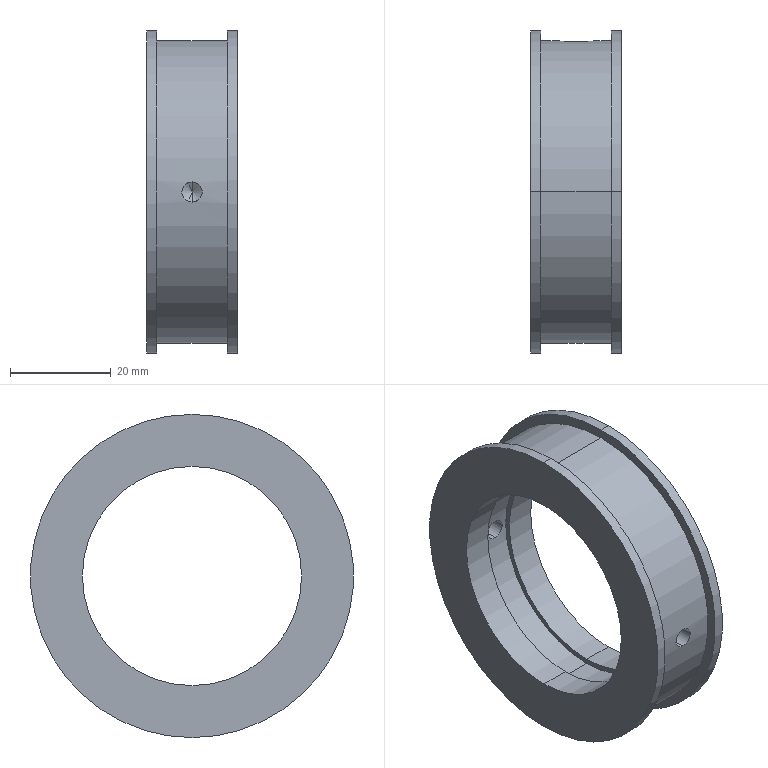Part | SolidWorks | features HoleWzd 3, Fillet 2, Revolution 1 | 1 solid | 31 faces | box 18 x 64 x 64 mm | volume 24795 mm3 | cylinder 18 | plane 7 | torus 2 | spline 2 | cone 2 | commonest cylinder face diameters 4 x4 43.4 x4 64 x4 7.5 x2 45.4 x2 60 x2
STEP:
#1=CARTESIAN_POINT('',(0.6103,28.8,3.75));
#2=VERTEX_POINT('',#1);
#3=CARTESIAN_POINT('',(0.6103,28.8,-3.75));
#4=VERTEX_POINT('',#3);
#5=CARTESIAN_POINT('',(0.6103,28.8,0.));
#6=DIRECTION('',(0.,-1.,0.));
#7=DIRECTION('',(0.,0.,-1.));
#8=AXIS2_PLACEMENT_3D('',#5,#6,#7);
#9=CIRCLE('',#8,3.75);
#10=EDGE_CURVE('',#2,#4,#9,.T.);
#11=ORIENTED_EDGE('',*,*,#10,.F.);
#12=CARTESIAN_POINT('',(0.6103,28.5,3.45));
#13=VERTEX_POINT('',#12);
#14=CARTESIAN_POINT('',(0.6103,28.8,3.45));
#15=DIRECTION('',(1.,0.,0.));
#16=DIRECTION('',(0.,0.,-1.));
#17=AXIS2_PLACEMENT_3D('',#14,#15,#16);
#18=CIRCLE('',#17,0.3);
#19=EDGE_CURVE('',#2,#13,#18,.T.);
#20=ORIENTED_EDGE('',*,*,#19,.T.);
#21=CARTESIAN_POINT('',(0.6103,28.5,-3.45));
#22=VERTEX_POINT('',#21);
#23=CARTESIAN_POINT('',(0.6103,28.5,0.));
#24=DIRECTION('',(0.,1.,0.));
#25=DIRECTION('',(0.,0.,-1.));
#26=AXIS2_PLACEMENT_3D('',#23,#24,#25);
#27=CIRCLE('',#26,3.45);
#28=EDGE_CURVE('',#22,#13,#27,.T.);
#29=ORIENTED_EDGE('',*,*,#28,.F.);
#30=CARTESIAN_POINT('',(0.6103,28.8,-3.45));
#31=DIRECTION('',(-1.,0.,0.));
#32=DIRECTION('',(0.,0.,1.));
#33=AXIS2_PLACEMENT_3D('',#30,#31,#32);
#34=CIRCLE('',#33,0.3);
#35=EDGE_CURVE('',#4,#22,#34,.T.);
#36=ORIENTED_EDGE('',*,*,#35,.F.);
#37=EDGE_LOOP('',(#11,#20,#29,#36));
#38=FACE_OUTER_BOUND('',#37,.T.);
#39=CARTESIAN_POINT('',(0.6103,28.8,0.));
#40=DIRECTION('',(0.,-1.,0.));
#41=DIRECTION('',(0.,0.,-1.));
#42=AXIS2_PLACEMENT_3D('',#39,#40,#41);
#43=TOROIDAL_SURFACE('',#42,3.45,0.3);
#44=ADVANCED_FACE('',(#38),#43,.F.);
#45=CARTESIAN_POINT('',(-0.2424,29.551,-3.652));
#46=VERTEX_POINT('',#45);
#47=CARTESIAN_POINT('',(0.6103,29.537,3.75));
#48=VERTEX_POINT('',#47);
#49=CARTESIAN_POINT('',(-0.2424,29.551,-3.652));
#50=CARTESIAN_POINT('',(-0.4646,29.558,-3.6));
#51=CARTESIAN_POINT('',(-0.6839,29.568,-3.527));
#52=CARTESIAN_POINT('',(-1.101,29.591,-3.345));
#53=CARTESIAN_POINT('',(-1.299,29.605,-3.236));
#54=CARTESIAN_POINT('',(-1.675,29.634,-2.982));
#55=CARTESIAN_POINT('',(-1.854,29.65,-2.836));
#56=CARTESIAN_POINT('',(-2.178,29.682,-2.518));
#57=CARTESIAN_POINT('',(-2.324,29.698,-2.346));
#58=CARTESIAN_POINT('',(-2.586,29.728,-1.974));
#59=CARTESIAN_POINT('',(-2.701,29.742,-1.774));
#60=CARTESIAN_POINT('',(-2.891,29.766,-1.363));
#61=CARTESIAN_POINT('',(-2.967,29.776,-1.149));
#62=CARTESIAN_POINT('',(-3.08,29.792,-0.7059));
#63=CARTESIAN_POINT('',(-3.116,29.797,-0.479));
#64=CARTESIAN_POINT('',(-3.146,29.801,-0.02683));
#65=CARTESIAN_POINT('',(-3.141,29.8,0.2003));
#66=CARTESIAN_POINT('',(-3.089,29.793,0.6567));
#67=CARTESIAN_POINT('',(-3.042,29.786,0.8794));
#68=CARTESIAN_POINT('',(-2.91,29.769,1.312));
#69=CARTESIAN_POINT('',(-2.823,29.757,1.524));
#70=CARTESIAN_POINT('',(-2.613,29.731,1.93));
#71=CARTESIAN_POINT('',(-2.491,29.717,2.121));
#72=CARTESIAN_POINT('',(-2.213,29.686,2.478));
#73=CARTESIAN_POINT('',(-2.056,29.67,2.647));
#74=CARTESIAN_POINT('',(-1.716,29.638,2.95));
#75=CARTESIAN_POINT('',(-1.534,29.623,3.084));
#76=CARTESIAN_POINT('',(-1.147,29.594,3.32));
#77=CARTESIAN_POINT('',(-0.9399,29.581,3.422));
#78=CARTESIAN_POINT('',(-0.5152,29.56,3.584));
#79=CARTESIAN_POINT('',(-0.2972,29.552,3.646));
#80=CARTESIAN_POINT('',(0.1503,29.54,3.729));
#81=CARTESIAN_POINT('',(0.3805,29.537,3.75));
#82=CARTESIAN_POINT('',(0.6103,29.537,3.75));
#83=B_SPLINE_CURVE_WITH_KNOTS('',3,(#49,#50,#51,#52,#53,#54,#55,#56,#57,#58,#59,#60,#61,#62,#63,#64,#65,#66,#67,#68,#69,#70,#71,#72,#73,#74,#75,#76,#77,#78,#79,#80,#81,#82),.UNSPECIFIED.,.F.,.F.,(4,2,2,2,2,2,2,2,2,2,2,2,2,2,2,2,4),(0.01269,0.01337,0.01406,0.01474,0.01543,0.01611,0.0168,0.01748,0.01817,0.01885,0.01954,0.02022,0.02091,0.02159,0.02228,0.02296,0.02365),.UNSPECIFIED.);
#84=EDGE_CURVE('',#46,#48,#83,.T.);
#85=ORIENTED_EDGE('',*,*,#84,.F.);
#86=CARTESIAN_POINT('',(-0.2879,29.749,-3.872));
#87=VERTEX_POINT('',#86);
#88=CARTESIAN_POINT('',(-0.2879,29.551,-3.847));
#89=DIRECTION('',(-0.9734,0.02959,0.2273));
#90=DIRECTION('',(0.2274,0.,0.9738));
#91=AXIS2_PLACEMENT_3D('',#88,#89,#90);
#92=CIRCLE('',#91,0.2);
#93=EDGE_CURVE('',#46,#87,#92,.T.);
#94=ORIENTED_EDGE('',*,*,#93,.T.);
#95=CARTESIAN_POINT('',(1.509,29.749,3.872));
#96=VERTEX_POINT('',#95);
#97=CARTESIAN_POINT('',(1.509,29.749,3.872));
#98=CARTESIAN_POINT('',(1.254,29.741,3.932));
#99=CARTESIAN_POINT('',(0.9958,29.737,3.966));
#100=CARTESIAN_POINT('',(0.4738,29.734,3.983));
#101=CARTESIAN_POINT('',(0.2098,29.737,3.965));
#102=CARTESIAN_POINT('',(-0.3023,29.748,3.878));
#103=CARTESIAN_POINT('',(-0.5513,29.757,3.81));
#104=CARTESIAN_POINT('',(-1.035,29.78,3.624));
#105=CARTESIAN_POINT('',(-1.271,29.795,3.506));
#106=CARTESIAN_POINT('',(-1.707,29.826,3.231));
#107=CARTESIAN_POINT('',(-1.911,29.843,3.072));
#108=CARTESIAN_POINT('',(-2.289,29.878,2.714));
#109=CARTESIAN_POINT('',(-2.459,29.895,2.517));
#110=CARTESIAN_POINT('',(-2.756,29.927,2.096));
#111=CARTESIAN_POINT('',(-2.886,29.943,1.869));
#112=CARTESIAN_POINT('',(-3.098,29.969,1.394));
#113=CARTESIAN_POINT('',(-3.18,29.979,1.149));
#114=CARTESIAN_POINT('',(-3.296,29.994,0.6447));
#115=CARTESIAN_POINT('',(-3.33,29.999,0.3829));
#116=CARTESIAN_POINT('',(-3.346,30.001,-0.135));
#117=CARTESIAN_POINT('',(-3.329,29.999,-0.3927));
#118=CARTESIAN_POINT('',(-3.245,29.987,-0.9056));
#119=CARTESIAN_POINT('',(-3.177,29.979,-1.16));
#120=CARTESIAN_POINT('',(-2.996,29.956,-1.643));
#121=CARTESIAN_POINT('',(-2.882,29.942,-1.876));
#122=CARTESIAN_POINT('',(-2.608,29.911,-2.321));
#123=CARTESIAN_POINT('',(-2.451,29.894,-2.526));
#124=CARTESIAN_POINT('',(-2.1,29.86,-2.904));
#125=CARTESIAN_POINT('',(-1.904,29.842,-3.078));
#126=CARTESIAN_POINT('',(-1.484,29.809,-3.382));
#127=CARTESIAN_POINT('',(-1.261,29.794,-3.512));
#128=CARTESIAN_POINT('',(-0.7903,29.768,-3.727));
#129=CARTESIAN_POINT('',(-0.5411,29.757,-3.813));
#130=CARTESIAN_POINT('',(-0.2879,29.749,-3.872));
#131=B_SPLINE_CURVE_WITH_KNOTS('',3,(#97,#98,#99,#100,#101,#102,#103,#104,#105,#106,#107,#108,#109,#110,#111,#112,#113,#114,#115,#116,#117,#118,#119,#120,#121,#122,#123,#124,#125,#126,#127,#128,#129,#130),.UNSPECIFIED.,.F.,.F.,(4,2,2,2,2,2,2,2,2,2,2,2,2,2,2,2,4),(0.02421,0.025,0.02578,0.02657,0.02735,0.02814,0.02892,0.02971,0.03049,0.03128,0.03206,0.03285,0.03363,0.03442,0.0352,0.03599,0.03677),.UNSPECIFIED.);
#132=EDGE_CURVE('',#96,#87,#131,.T.);
#133=ORIENTED_EDGE('',*,*,#132,.F.);
#134=CARTESIAN_POINT('',(1.463,29.551,3.652));
#135=VERTEX_POINT('',#134);
#136=CARTESIAN_POINT('',(1.509,29.551,3.846));
#137=DIRECTION('',(0.9734,0.02959,-0.2273));
#138=DIRECTION('',(-0.2274,0.,-0.9738));
#139=AXIS2_PLACEMENT_3D('',#136,#137,#138);
#140=CIRCLE('',#139,0.2);
#141=EDGE_CURVE('',#135,#96,#140,.T.);
#142=ORIENTED_EDGE('',*,*,#141,.F.);
#143=CARTESIAN_POINT('',(0.6103,29.537,3.75));
#144=CARTESIAN_POINT('',(0.7544,29.537,3.75));
#145=CARTESIAN_POINT('',(1.041,29.539,3.733));
#146=CARTESIAN_POINT('',(1.323,29.546,3.684));
#147=CARTESIAN_POINT('',(1.463,29.551,3.652));
#148=B_SPLINE_CURVE_WITH_KNOTS('',3,(#143,#144,#145,#146,#147),.UNSPECIFIED.,.F.,.F.,(4,1,4),(0.,0.0004293,0.0008586),.UNSPECIFIED.);
#149=EDGE_CURVE('',#48,#135,#148,.T.);
#150=ORIENTED_EDGE('',*,*,#149,.F.);
#151=EDGE_LOOP('',(#85,#94,#133,#142,#150));
#152=FACE_OUTER_BOUND('',#151,.T.);
#153=CARTESIAN_POINT('',(1.463,29.551,3.652));
#154=CARTESIAN_POINT('',(1.457,29.778,3.653));
#155=CARTESIAN_POINT('',(1.509,29.749,3.872));
#156=CARTESIAN_POINT('',(1.222,29.543,3.708));
#157=CARTESIAN_POINT('',(1.216,29.771,3.709));
#158=CARTESIAN_POINT('',(1.254,29.741,3.932));
#159=CARTESIAN_POINT('',(0.9788,29.538,3.74));
#160=CARTESIAN_POINT('',(0.9757,29.767,3.74));
#161=CARTESIAN_POINT('',(0.9985,29.737,3.966));
#162=CARTESIAN_POINT('',(0.49,29.536,3.756));
#163=CARTESIAN_POINT('',(0.4909,29.765,3.756));
#164=CARTESIAN_POINT('',(0.4835,29.734,3.983));
#165=CARTESIAN_POINT('',(0.2413,29.539,3.74));
#166=CARTESIAN_POINT('',(0.2448,29.767,3.74));
#167=CARTESIAN_POINT('',(0.2217,29.737,3.966));
#168=CARTESIAN_POINT('',(-0.2441,29.55,3.66));
#169=CARTESIAN_POINT('',(-0.237,29.777,3.661));
#170=CARTESIAN_POINT('',(-0.2896,29.748,3.881));
#171=CARTESIAN_POINT('',(-0.4801,29.558,3.596));
#172=CARTESIAN_POINT('',(-0.4712,29.784,3.599));
#173=CARTESIAN_POINT('',(-0.5383,29.757,3.814));
#174=CARTESIAN_POINT('',(-0.9391,29.581,3.424));
#175=CARTESIAN_POINT('',(-0.928,29.804,3.429));
#176=CARTESIAN_POINT('',(-1.022,29.78,3.631));
#177=CARTESIAN_POINT('',(-1.163,29.595,3.313));
#178=CARTESIAN_POINT('',(-1.151,29.817,3.32));
#179=CARTESIAN_POINT('',(-1.257,29.794,3.513));
#180=CARTESIAN_POINT('',(-1.578,29.626,3.055));
#181=CARTESIAN_POINT('',(-1.566,29.844,3.064));
#182=CARTESIAN_POINT('',(-1.695,29.825,3.24));
#183=CARTESIAN_POINT('',(-1.772,29.643,2.907));
#184=CARTESIAN_POINT('',(-1.76,29.859,2.916));
#185=CARTESIAN_POINT('',(-1.899,29.842,3.082));
#186=CARTESIAN_POINT('',(-2.132,29.677,2.57));
#187=CARTESIAN_POINT('',(-2.121,29.89,2.581));
#188=CARTESIAN_POINT('',(-2.278,29.877,2.725));
#189=CARTESIAN_POINT('',(-2.294,29.695,2.384));
#190=CARTESIAN_POINT('',(-2.285,29.905,2.396));
#191=CARTESIAN_POINT('',(-2.449,29.894,2.528));
#192=CARTESIAN_POINT('',(-2.579,29.727,1.988));
#193=CARTESIAN_POINT('',(-2.572,29.934,1.999));
#194=CARTESIAN_POINT('',(-2.749,29.927,2.108));
#195=CARTESIAN_POINT('',(-2.703,29.742,1.774));
#196=CARTESIAN_POINT('',(-2.697,29.948,1.785));
#197=CARTESIAN_POINT('',(-2.88,29.942,1.881));
#198=CARTESIAN_POINT('',(-2.907,29.768,1.325));
#199=CARTESIAN_POINT('',(-2.903,29.971,1.334));
#200=CARTESIAN_POINT('',(-3.094,29.968,1.405));
#201=CARTESIAN_POINT('',(-2.985,29.779,1.093));
#202=CARTESIAN_POINT('',(-2.983,29.981,1.101));
#203=CARTESIAN_POINT('',(-3.177,29.979,1.159));
#204=CARTESIAN_POINT('',(-3.097,29.794,0.6165));
#205=CARTESIAN_POINT('',(-3.096,29.995,0.6213));
#206=CARTESIAN_POINT('',(-3.294,29.994,0.6537));
#207=CARTESIAN_POINT('',(-3.13,29.799,0.3687));
#208=CARTESIAN_POINT('',(-3.129,29.999,0.3714));
#209=CARTESIAN_POINT('',(-3.329,29.999,0.391));
#210=CARTESIAN_POINT('',(-3.146,29.801,-0.1217));
#211=CARTESIAN_POINT('',(-3.146,30.001,-0.1225));
#212=CARTESIAN_POINT('',(-3.346,30.001,-0.129));
#213=CARTESIAN_POINT('',(-3.13,29.799,-0.3657));
#214=CARTESIAN_POINT('',(-3.13,29.999,-0.3686));
#215=CARTESIAN_POINT('',(-3.329,29.999,-0.3878));
#216=CARTESIAN_POINT('',(-3.05,29.788,-0.8512));
#217=CARTESIAN_POINT('',(-3.049,29.989,-0.8574));
#218=CARTESIAN_POINT('',(-3.245,29.988,-0.9027));
#219=CARTESIAN_POINT('',(-2.986,29.779,-1.092));
#220=CARTESIAN_POINT('',(-2.983,29.981,-1.1));
#221=CARTESIAN_POINT('',(-3.177,29.979,-1.158));
#222=CARTESIAN_POINT('',(-2.813,29.756,-1.549));
#223=CARTESIAN_POINT('',(-2.809,29.96,-1.559));
#224=CARTESIAN_POINT('',(-2.996,29.956,-1.643));
#225=CARTESIAN_POINT('',(-2.705,29.743,-1.769));
#226=CARTESIAN_POINT('',(-2.699,29.948,-1.78));
#227=CARTESIAN_POINT('',(-2.882,29.942,-1.876));
#228=CARTESIAN_POINT('',(-2.444,29.711,-2.189));
#229=CARTESIAN_POINT('',(-2.436,29.92,-2.201));
#230=CARTESIAN_POINT('',(-2.607,29.911,-2.322));
#231=CARTESIAN_POINT('',(-2.295,29.695,-2.383));
#232=CARTESIAN_POINT('',(-2.286,29.905,-2.395));
#233=CARTESIAN_POINT('',(-2.45,29.894,-2.527));
#234=CARTESIAN_POINT('',(-1.962,29.661,-2.74));
#235=CARTESIAN_POINT('',(-1.95,29.875,-2.751));
#236=CARTESIAN_POINT('',(-2.099,29.86,-2.905));
#237=CARTESIAN_POINT('',(-1.775,29.643,-2.904));
#238=CARTESIAN_POINT('',(-1.763,29.859,-2.914));
#239=CARTESIAN_POINT('',(-1.902,29.842,-3.08));
#240=CARTESIAN_POINT('',(-1.376,29.61,-3.19));
#241=CARTESIAN_POINT('',(-1.364,29.83,-3.198));
#242=CARTESIAN_POINT('',(-1.482,29.809,-3.383));
#243=CARTESIAN_POINT('',(-1.165,29.595,-3.312));
#244=CARTESIAN_POINT('',(-1.153,29.817,-3.319));
#245=CARTESIAN_POINT('',(-1.259,29.794,-3.512));
#246=CARTESIAN_POINT('',(-0.7184,29.569,-3.515));
#247=CARTESIAN_POINT('',(-0.7081,29.794,-3.519));
#248=CARTESIAN_POINT('',(-0.7893,29.768,-3.728));
#249=CARTESIAN_POINT('',(-0.4816,29.558,-3.596));
#250=CARTESIAN_POINT('',(-0.4729,29.784,-3.598));
#251=CARTESIAN_POINT('',(-0.5398,29.757,-3.813));
#252=CARTESIAN_POINT('',(-0.2424,29.551,-3.652));
#253=CARTESIAN_POINT('',(-0.2359,29.778,-3.653));
#254=CARTESIAN_POINT('',(-0.2879,29.749,-3.872));
#255=(BOUNDED_SURFACE()B_SPLINE_SURFACE(3,2,((#153,#154,#155),(#156,#157,#158),(#159,#160,#161),(#162,#163,#164),(#165,#166,#167),(#168,#169,#170),(#171,#172,#173),(#174,#175,#176),(#177,#178,#179),(#180,#181,#182),(#183,#184,#185),(#186,#187,#188),(#189,#190,#191),(#192,#193,#194),(#195,#196,#197),(#198,#199,#200),(#201,#202,#203),(#204,#205,#206),(#207,#208,#209),(#210,#211,#212),(#213,#214,#215),(#216,#217,#218),(#219,#220,#221),(#222,#223,#224),(#225,#226,#227),(#228,#229,#230),(#231,#232,#233),(#234,#235,#236),(#237,#238,#239),(#240,#241,#242),(#243,#244,#245),(#246,#247,#248),(#249,#250,#251),(#252,#253,#254)),.UNSPECIFIED.,.F.,.F.,.T.)B_SPLINE_SURFACE_WITH_KNOTS((4,2,2,2,2,2,2,2,2,2,2,2,2,2,2,2,4),(3,3),(0.,0.0007725,0.001545,0.002318,0.00309,0.003863,0.004635,0.005408,0.00618,0.006953,0.007725,0.008498,0.00927,0.01004,0.01082,0.01159,0.01236),(0.,1.),.UNSPECIFIED.)GEOMETRIC_REPRESENTATION_ITEM()RATIONAL_B_SPLINE_SURFACE(((1.,0.6612,1.),(1.,0.6597,1.),(1.,0.6588,1.),(1.,0.6584,1.),(1.,0.6589,1.),(1.,0.661,1.),(1.,0.6626,1.),(1.,0.6669,1.),(1.,0.6696,1.),(1.,0.6754,1.),(1.,0.6785,1.),(1.,0.6849,1.),(1.,0.688,1.),(1.,0.694,1.),(1.,0.6967,1.),(1.,0.7014,1.),(1.,0.7033,1.),(1.,0.706,1.),(1.,0.7069,1.),(1.,0.7073,1.),(1.,0.7069,1.),(1.,0.7049,1.),(1.,0.7033,1.),(1.,0.6992,1.),(1.,0.6968,1.),(1.,0.6911,1.),(1.,0.688,1.),(1.,0.6817,1.),(1.,0.6785,1.),(1.,0.6724,1.),(1.,0.6696,1.),(1.,0.6647,1.),(1.,0.6626,1.),(1.,0.6612,1.)))REPRESENTATION_ITEM('')SURFACE());
#256=ADVANCED_FACE('',(#152),#255,.T.);
#257=CARTESIAN_POINT('',(0.6103,-24.798,0.));
#258=VERTEX_POINT('',#257);
#259=CARTESIAN_POINT('',(0.6103,-26.,-2.));
#260=VERTEX_POINT('',#259);
#261=CARTESIAN_POINT('',(0.6103,-26.,-2.));
#262=DIRECTION('',(0.,-0.515,-0.8572));
#263=VECTOR('',#262,1000.);
#264=LINE('',#261,#263);
#265=EDGE_CURVE('',#258,#260,#264,.T.);
#266=ORIENTED_EDGE('',*,*,#265,.F.);
#267=CARTESIAN_POINT('',(0.6103,-26.,2.));
#268=VERTEX_POINT('',#267);
#269=CARTESIAN_POINT('',(0.6103,-26.,2.));
#270=DIRECTION('',(0.,-0.515,0.8572));
#271=VECTOR('',#270,1000.);
#272=LINE('',#269,#271);
#273=EDGE_CURVE('',#258,#268,#272,.T.);
#274=ORIENTED_EDGE('',*,*,#273,.T.);
#275=CARTESIAN_POINT('',(0.6103,-26.,0.));
#276=DIRECTION('',(0.,-1.,0.));
#277=DIRECTION('',(0.,0.,-1.));
#278=AXIS2_PLACEMENT_3D('',#275,#276,#277);
#279=CIRCLE('',#278,2.);
#280=EDGE_CURVE('',#268,#260,#279,.T.);
#281=ORIENTED_EDGE('',*,*,#280,.T.);
#282=EDGE_LOOP('',(#266,#274,#281));
#283=FACE_OUTER_BOUND('',#282,.T.);
#284=CARTESIAN_POINT('',(0.6103,-26.,0.));
#285=DIRECTION('',(0.,-1.,0.));
#286=DIRECTION('',(0.,0.,-1.));
#287=AXIS2_PLACEMENT_3D('',#284,#285,#286);
#288=CONICAL_SURFACE('',#287,2.,1.03);
#289=ADVANCED_FACE('',(#283),#288,.F.);
#290=ORIENTED_EDGE('',*,*,#280,.F.);
#291=CARTESIAN_POINT('',(0.6103,-29.933,2.));
#292=VERTEX_POINT('',#291);
#293=CARTESIAN_POINT('',(0.6103,-30.,2.));
#294=DIRECTION('',(0.,-1.,0.));
#295=VECTOR('',#294,1000.);
#296=LINE('',#293,#295);
#297=EDGE_CURVE('',#268,#292,#296,.T.);
#298=ORIENTED_EDGE('',*,*,#297,.T.);
#299=CARTESIAN_POINT('',(0.6103,-29.933,-2.));
#300=VERTEX_POINT('',#299);
#301=CARTESIAN_POINT('',(0.6103,-29.933,-2.));
#302=CARTESIAN_POINT('',(0.4782,-29.933,-2.));
#303=CARTESIAN_POINT('',(0.3482,-29.934,-1.987));
#304=CARTESIAN_POINT('',(0.0925,-29.937,-1.936));
#305=CARTESIAN_POINT('',(-0.03454,-29.94,-1.898));
#306=CARTESIAN_POINT('',(-0.2768,-29.946,-1.797));
#307=CARTESIAN_POINT('',(-0.3916,-29.95,-1.736));
#308=CARTESIAN_POINT('',(-0.609,-29.958,-1.591));
#309=CARTESIAN_POINT('',(-0.7119,-29.962,-1.506));
#310=CARTESIAN_POINT('',(-0.9886,-29.975,-1.229));
#311=CARTESIAN_POINT('',(-1.138,-29.984,-1.006));
#312=CARTESIAN_POINT('',(-1.337,-29.996,-0.525));
#313=CARTESIAN_POINT('',(-1.39,-30.,-0.2617));
#314=CARTESIAN_POINT('',(-1.39,-30.,0.1298));
#315=CARTESIAN_POINT('',(-1.377,-29.999,0.2623));
#316=CARTESIAN_POINT('',(-1.326,-29.996,0.5189));
#317=CARTESIAN_POINT('',(-1.288,-29.993,0.6436));
#318=CARTESIAN_POINT('',(-1.188,-29.987,0.8858));
#319=CARTESIAN_POINT('',(-1.125,-29.983,1.003));
#320=CARTESIAN_POINT('',(-0.9802,-29.975,1.22));
#321=CARTESIAN_POINT('',(-0.8975,-29.971,1.321));
#322=CARTESIAN_POINT('',(-0.7108,-29.962,1.507));
#323=CARTESIAN_POINT('',(-0.6097,-29.958,1.59));
#324=CARTESIAN_POINT('',(-0.3931,-29.95,1.735));
#325=CARTESIAN_POINT('',(-0.2762,-29.946,1.798));
#326=CARTESIAN_POINT('',(-0.03384,-29.94,1.898));
#327=CARTESIAN_POINT('',(0.09085,-29.937,1.936));
#328=CARTESIAN_POINT('',(0.3472,-29.934,1.987));
#329=CARTESIAN_POINT('',(0.4798,-29.933,2.));
#330=CARTESIAN_POINT('',(0.6103,-29.933,2.));
#331=B_SPLINE_CURVE_WITH_KNOTS('',3,(#301,#302,#303,#304,#305,#306,#307,#308,#309,#310,#311,#312,#313,#314,#315,#316,#317,#318,#319,#320,#321,#322,#323,#324,#325,#326,#327,#328,#329,#330),.UNSPECIFIED.,.F.,.F.,(4,2,2,2,2,2,2,2,2,2,2,2,2,2,4),(0.,0.0003909,0.0007818,0.001173,0.001564,0.002345,0.003127,0.003518,0.003909,0.0043,0.004691,0.005082,0.005473,0.005864,0.006255),.UNSPECIFIED.);
#332=EDGE_CURVE('',#300,#292,#331,.T.);
#333=ORIENTED_EDGE('',*,*,#332,.F.);
#334=CARTESIAN_POINT('',(0.6103,-30.,-2.));
#335=DIRECTION('',(0.,-1.,0.));
#336=VECTOR('',#335,1000.);
#337=LINE('',#334,#336);
#338=EDGE_CURVE('',#260,#300,#337,.T.);
#339=ORIENTED_EDGE('',*,*,#338,.F.);
#340=EDGE_LOOP('',(#290,#298,#333,#339));
#341=FACE_OUTER_BOUND('',#340,.T.);
#342=CARTESIAN_POINT('',(0.6103,-30.,0.));
#343=DIRECTION('',(0.,-1.,0.));
#344=DIRECTION('',(0.,0.,-1.));
#345=AXIS2_PLACEMENT_3D('',#342,#343,#344);
#346=CYLINDRICAL_SURFACE('',#345,2.);
#347=ADVANCED_FACE('',(#341),#346,.F.);
#348=CARTESIAN_POINT('',(0.6103,22.612,-2.));
#349=VERTEX_POINT('',#348);
#350=CARTESIAN_POINT('',(0.6103,22.612,2.));
#351=VERTEX_POINT('',#350);
#352=CARTESIAN_POINT('',(0.6103,22.612,-2.));
#353=CARTESIAN_POINT('',(0.3493,22.612,-2.));
#354=CARTESIAN_POINT('',(0.08608,22.617,-1.948));
#355=CARTESIAN_POINT('',(-0.3953,22.633,-1.748));
#356=CARTESIAN_POINT('',(-0.6184,22.644,-1.599));
#357=CARTESIAN_POINT('',(-0.8951,22.662,-1.323));
#358=CARTESIAN_POINT('',(-0.9796,22.667,-1.22));
#359=CARTESIAN_POINT('',(-1.125,22.678,-1.003));
#360=CARTESIAN_POINT('',(-1.186,22.683,-0.8882));
#361=CARTESIAN_POINT('',(-1.287,22.691,-0.6463));
#362=CARTESIAN_POINT('',(-1.325,22.694,-0.5192));
#363=CARTESIAN_POINT('',(-1.377,22.699,-0.2635));
#364=CARTESIAN_POINT('',(-1.39,22.7,-0.1336));
#365=CARTESIAN_POINT('',(-1.39,22.7,0.1305));
#366=CARTESIAN_POINT('',(-1.377,22.699,0.2608));
#367=CARTESIAN_POINT('',(-1.326,22.694,0.5164));
#368=CARTESIAN_POINT('',(-1.288,22.691,0.6434));
#369=CARTESIAN_POINT('',(-1.188,22.683,0.8857));
#370=CARTESIAN_POINT('',(-1.126,22.678,1.001));
#371=CARTESIAN_POINT('',(-0.9814,22.668,1.218));
#372=CARTESIAN_POINT('',(-0.897,22.662,1.321));
#373=CARTESIAN_POINT('',(-0.6205,22.644,1.598));
#374=CARTESIAN_POINT('',(-0.3977,22.633,1.747));
#375=CARTESIAN_POINT('',(0.08333,22.617,1.947));
#376=CARTESIAN_POINT('',(0.346,22.612,2.));
#377=CARTESIAN_POINT('',(0.6103,22.612,2.));
#378=B_SPLINE_CURVE_WITH_KNOTS('',3,(#352,#353,#354,#355,#356,#357,#358,#359,#360,#361,#362,#363,#364,#365,#366,#367,#368,#369,#370,#371,#372,#373,#374,#375,#376,#377),.UNSPECIFIED.,.F.,.F.,(4,2,2,2,2,2,2,2,2,2,2,2,4),(0.006256,0.007038,0.00782,0.00821,0.008601,0.008992,0.009383,0.009774,0.01016,0.01056,0.01095,0.01173,0.01251),.UNSPECIFIED.);
#379=EDGE_CURVE('',#349,#351,#378,.T.);
#380=ORIENTED_EDGE('',*,*,#379,.F.);
#381=CARTESIAN_POINT('',(0.6103,28.5,-2.));
#382=VERTEX_POINT('',#381);
#383=CARTESIAN_POINT('',(0.6103,28.5,-2.));
#384=DIRECTION('',(0.,1.,0.));
#385=VECTOR('',#384,1000.);
#386=LINE('',#383,#385);
#387=EDGE_CURVE('',#349,#382,#386,.T.);
#388=ORIENTED_EDGE('',*,*,#387,.T.);
#389=CARTESIAN_POINT('',(0.6103,28.5,2.));
#390=VERTEX_POINT('',#389);
#391=CARTESIAN_POINT('',(0.6103,28.5,0.));
#392=DIRECTION('',(0.,1.,0.));
#393=DIRECTION('',(0.,0.,1.));
#394=AXIS2_PLACEMENT_3D('',#391,#392,#393);
#395=CIRCLE('',#394,2.);
#396=EDGE_CURVE('',#382,#390,#395,.T.);
#397=ORIENTED_EDGE('',*,*,#396,.T.);
#398=CARTESIAN_POINT('',(0.6103,28.5,2.));
#399=DIRECTION('',(0.,1.,0.));
#400=VECTOR('',#399,1000.);
#401=LINE('',#398,#400);
#402=EDGE_CURVE('',#351,#390,#401,.T.);
#403=ORIENTED_EDGE('',*,*,#402,.F.);
#404=EDGE_LOOP('',(#380,#388,#397,#403));
#405=FACE_OUTER_BOUND('',#404,.T.);
#406=CARTESIAN_POINT('',(0.6103,28.5,0.));
#407=DIRECTION('',(0.,1.,0.));
#408=DIRECTION('',(0.,0.,1.));
#409=AXIS2_PLACEMENT_3D('',#406,#407,#408);
#410=CYLINDRICAL_SURFACE('',#409,2.);
#411=ADVANCED_FACE('',(#405),#410,.F.);
#412=ORIENTED_EDGE('',*,*,#10,.T.);
#413=CARTESIAN_POINT('',(0.6103,29.537,-3.75));
#414=VERTEX_POINT('',#413);
#415=CARTESIAN_POINT('',(0.6103,30.,-3.75));
#416=DIRECTION('',(0.,1.,0.));
#417=VECTOR('',#416,1000.);
#418=LINE('',#415,#417);
#419=EDGE_CURVE('',#4,#414,#418,.T.);
#420=ORIENTED_EDGE('',*,*,#419,.T.);
#421=CARTESIAN_POINT('',(0.6103,29.537,-3.75));
#422=CARTESIAN_POINT('',(0.4679,29.537,-3.75));
#423=CARTESIAN_POINT('',(0.325,29.538,-3.742));
#424=CARTESIAN_POINT('',(0.03842,29.543,-3.709));
#425=CARTESIAN_POINT('',(-0.1029,29.546,-3.684));
#426=CARTESIAN_POINT('',(-0.2424,29.551,-3.652));
#427=B_SPLINE_CURVE_WITH_KNOTS('',3,(#421,#422,#423,#424,#425,#426),.UNSPECIFIED.,.F.,.F.,(4,2,4),(0.01183,0.01226,0.01269),.UNSPECIFIED.);
#428=EDGE_CURVE('',#414,#46,#427,.T.);
#429=ORIENTED_EDGE('',*,*,#428,.T.);
#430=ORIENTED_EDGE('',*,*,#84,.T.);
#431=CARTESIAN_POINT('',(0.6103,30.,3.75));
#432=DIRECTION('',(0.,1.,0.));
#433=VECTOR('',#432,1000.);
#434=LINE('',#431,#433);
#435=EDGE_CURVE('',#2,#48,#434,.T.);
#436=ORIENTED_EDGE('',*,*,#435,.F.);
#437=EDGE_LOOP('',(#412,#420,#429,#430,#436));
#438=FACE_OUTER_BOUND('',#437,.T.);
#439=CARTESIAN_POINT('',(0.6103,30.,0.));
#440=DIRECTION('',(0.,1.,0.));
#441=DIRECTION('',(0.,0.,1.));
#442=AXIS2_PLACEMENT_3D('',#439,#440,#441);
#443=CYLINDRICAL_SURFACE('',#442,3.75);
#444=ADVANCED_FACE('',(#438),#443,.F.);
#445=CARTESIAN_POINT('',(-2.39,0.,-21.7));
#446=VERTEX_POINT('',#445);
#447=CARTESIAN_POINT('',(-2.39,0.,21.7));
#448=VERTEX_POINT('',#447);
#449=CARTESIAN_POINT('',(-2.39,0.,0.));
#450=DIRECTION('',(-1.,0.,0.));
#451=DIRECTION('',(0.,0.,1.));
#452=AXIS2_PLACEMENT_3D('',#449,#450,#451);
#453=CIRCLE('',#452,21.7);
#454=EDGE_CURVE('',#446,#448,#453,.T.);
#455=ORIENTED_EDGE('',*,*,#454,.F.);
#456=CARTESIAN_POINT('',(-8.39,0.,-21.7));
#457=VERTEX_POINT('',#456);
#458=CARTESIAN_POINT('',(-19.037,0.,-21.7));
#459=DIRECTION('',(-1.,0.,0.));
#460=VECTOR('',#459,1000.);
#461=LINE('',#458,#460);
#462=EDGE_CURVE('',#446,#457,#461,.T.);
#463=ORIENTED_EDGE('',*,*,#462,.T.);
#464=CARTESIAN_POINT('',(-8.39,0.,21.7));
#465=VERTEX_POINT('',#464);
#466=CARTESIAN_POINT('',(-8.39,0.,0.));
#467=DIRECTION('',(-1.,0.,0.));
#468=DIRECTION('',(0.,0.,1.));
#469=AXIS2_PLACEMENT_3D('',#466,#467,#468);
#470=CIRCLE('',#469,21.7);
#471=EDGE_CURVE('',#457,#465,#470,.T.);
#472=ORIENTED_EDGE('',*,*,#471,.T.);
#473=CARTESIAN_POINT('',(-19.037,0.,21.7));
#474=DIRECTION('',(-1.,0.,0.));
#475=VECTOR('',#474,1000.);
#476=LINE('',#473,#475);
#477=EDGE_CURVE('',#448,#465,#476,.T.);
#478=ORIENTED_EDGE('',*,*,#477,.F.);
#479=EDGE_LOOP('',(#455,#463,#472,#478));
#480=FACE_OUTER_BOUND('',#479,.T.);
#481=CARTESIAN_POINT('',(-19.037,0.,0.));
#482=DIRECTION('',(-1.,0.,0.));
#483=DIRECTION('',(0.,0.,1.));
#484=AXIS2_PLACEMENT_3D('',#481,#482,#483);
#485=CYLINDRICAL_SURFACE('',#484,21.7);
#486=ADVANCED_FACE('',(#480),#485,.F.);
#487=CARTESIAN_POINT('',(3.61,0.,-22.7));
#488=VERTEX_POINT('',#487);
#489=CARTESIAN_POINT('',(3.61,0.,22.7));
#490=VERTEX_POINT('',#489);
#491=CARTESIAN_POINT('',(3.61,0.,0.));
#492=DIRECTION('',(-1.,0.,0.));
#493=DIRECTION('',(0.,0.,1.));
#494=AXIS2_PLACEMENT_3D('',#491,#492,#493);
#495=CIRCLE('',#494,22.7);
#496=EDGE_CURVE('',#488,#490,#495,.T.);
#497=ORIENTED_EDGE('',*,*,#496,.F.);
#498=CARTESIAN_POINT('',(-2.39,0.,-22.7));
#499=VERTEX_POINT('',#498);
#500=CARTESIAN_POINT('',(-19.037,0.,-22.7));
#501=DIRECTION('',(-1.,0.,0.));
#502=VECTOR('',#501,1000.);
#503=LINE('',#500,#502);
#504=EDGE_CURVE('',#488,#499,#503,.T.);
#505=ORIENTED_EDGE('',*,*,#504,.T.);
#506=CARTESIAN_POINT('',(-2.39,0.,22.7));
#507=VERTEX_POINT('',#506);
#508=CARTESIAN_POINT('',(-2.39,0.,0.));
#509=DIRECTION('',(-1.,0.,0.));
#510=DIRECTION('',(0.,0.,1.));
#511=AXIS2_PLACEMENT_3D('',#508,#509,#510);
#512=CIRCLE('',#511,22.7);
#513=EDGE_CURVE('',#499,#507,#512,.T.);
#514=ORIENTED_EDGE('',*,*,#513,.T.);
#515=CARTESIAN_POINT('',(-19.037,0.,22.7));
#516=DIRECTION('',(-1.,0.,0.));
#517=VECTOR('',#516,1000.);
#518=LINE('',#515,#517);
#519=EDGE_CURVE('',#490,#507,#518,.T.);
#520=ORIENTED_EDGE('',*,*,#519,.F.);
#521=EDGE_LOOP('',(#497,#505,#514,#520));
#522=FACE_OUTER_BOUND('',#521,.T.);
#523=CARTESIAN_POINT('',(-19.037,0.,0.));
#524=DIRECTION('',(-1.,0.,0.));
#525=DIRECTION('',(0.,0.,1.));
#526=AXIS2_PLACEMENT_3D('',#523,#524,#525);
#527=CYLINDRICAL_SURFACE('',#526,22.7);
#528=ADVANCED_FACE('',(#522),#527,.F.);
#529=CARTESIAN_POINT('',(9.61,0.,-21.7));
#530=VERTEX_POINT('',#529);
#531=CARTESIAN_POINT('',(9.61,0.,21.7));
#532=VERTEX_POINT('',#531);
#533=CARTESIAN_POINT('',(9.61,0.,0.));
#534=DIRECTION('',(-1.,0.,0.));
#535=DIRECTION('',(0.,0.,1.));
#536=AXIS2_PLACEMENT_3D('',#533,#534,#535);
#537=CIRCLE('',#536,21.7);
#538=EDGE_CURVE('',#530,#532,#537,.T.);
#539=ORIENTED_EDGE('',*,*,#538,.F.);
#540=CARTESIAN_POINT('',(3.61,0.,-21.7));
#541=VERTEX_POINT('',#540);
#542=CARTESIAN_POINT('',(-19.037,0.,-21.7));
#543=DIRECTION('',(-1.,0.,0.));
#544=VECTOR('',#543,1000.);
#545=LINE('',#542,#544);
#546=EDGE_CURVE('',#530,#541,#545,.T.);
#547=ORIENTED_EDGE('',*,*,#546,.T.);
#548=CARTESIAN_POINT('',(3.61,0.,21.7));
#549=VERTEX_POINT('',#548);
#550=CARTESIAN_POINT('',(3.61,0.,0.));
#551=DIRECTION('',(-1.,0.,0.));
#552=DIRECTION('',(0.,0.,1.));
#553=AXIS2_PLACEMENT_3D('',#550,#551,#552);
#554=CIRCLE('',#553,21.7);
#555=EDGE_CURVE('',#541,#549,#554,.T.);
#556=ORIENTED_EDGE('',*,*,#555,.T.);
#557=CARTESIAN_POINT('',(-19.037,0.,21.7));
#558=DIRECTION('',(-1.,0.,0.));
#559=VECTOR('',#558,1000.);
#560=LINE('',#557,#559);
#561=EDGE_CURVE('',#532,#549,#560,.T.);
#562=ORIENTED_EDGE('',*,*,#561,.F.);
#563=EDGE_LOOP('',(#539,#547,#556,#562));
#564=FACE_OUTER_BOUND('',#563,.T.);
#565=CARTESIAN_POINT('',(-19.037,0.,0.));
#566=DIRECTION('',(-1.,0.,0.));
#567=DIRECTION('',(0.,0.,1.));
#568=AXIS2_PLACEMENT_3D('',#565,#566,#567);
#569=CYLINDRICAL_SURFACE('',#568,21.7);
#570=ADVANCED_FACE('',(#564),#569,.F.);
#571=CARTESIAN_POINT('',(9.61,0.,32.));
#572=VERTEX_POINT('',#571);
#573=CARTESIAN_POINT('',(9.61,0.,-32.));
#574=VERTEX_POINT('',#573);
#575=CARTESIAN_POINT('',(9.61,0.,0.));
#576=DIRECTION('',(-1.,0.,0.));
#577=DIRECTION('',(0.,0.,1.));
#578=AXIS2_PLACEMENT_3D('',#575,#576,#577);
#579=CIRCLE('',#578,32.);
#580=EDGE_CURVE('',#572,#574,#579,.T.);
#581=ORIENTED_EDGE('',*,*,#580,.T.);
#582=CARTESIAN_POINT('',(7.61,0.,-32.));
#583=VERTEX_POINT('',#582);
#584=CARTESIAN_POINT('',(-19.037,0.,-32.));
#585=DIRECTION('',(-1.,0.,0.));
#586=VECTOR('',#585,1000.);
#587=LINE('',#584,#586);
#588=EDGE_CURVE('',#574,#583,#587,.T.);
#589=ORIENTED_EDGE('',*,*,#588,.T.);
#590=CARTESIAN_POINT('',(7.61,0.,32.));
#591=VERTEX_POINT('',#590);
#592=CARTESIAN_POINT('',(7.61,0.,0.));
#593=DIRECTION('',(-1.,0.,0.));
#594=DIRECTION('',(0.,0.,1.));
#595=AXIS2_PLACEMENT_3D('',#592,#593,#594);
#596=CIRCLE('',#595,32.);
#597=EDGE_CURVE('',#591,#583,#596,.T.);
#598=ORIENTED_EDGE('',*,*,#597,.F.);
#599=CARTESIAN_POINT('',(-19.037,0.,32.));
#600=DIRECTION('',(-1.,0.,0.));
#601=VECTOR('',#600,1000.);
#602=LINE('',#599,#601);
#603=EDGE_CURVE('',#572,#591,#602,.T.);
#604=ORIENTED_EDGE('',*,*,#603,.F.);
#605=EDGE_LOOP('',(#581,#589,#598,#604));
#606=FACE_OUTER_BOUND('',#605,.T.);
#607=CARTESIAN_POINT('',(-19.037,0.,0.));
#608=DIRECTION('',(-1.,0.,0.));
#609=DIRECTION('',(0.,0.,1.));
#610=AXIS2_PLACEMENT_3D('',#607,#608,#609);
#611=CYLINDRICAL_SURFACE('',#610,32.);
#612=ADVANCED_FACE('',(#606),#611,.T.);
#613=ORIENTED_EDGE('',*,*,#132,.T.);
#614=CARTESIAN_POINT('',(-0.2879,29.749,-3.872));
#615=CARTESIAN_POINT('',(-0.03455,29.741,-3.932));
#616=CARTESIAN_POINT('',(0.2272,29.737,-3.966));
#617=CARTESIAN_POINT('',(0.7456,29.734,-3.983));
#618=CARTESIAN_POINT('',(1.003,29.737,-3.965));
#619=CARTESIAN_POINT('',(1.516,29.748,-3.879));
#620=CARTESIAN_POINT('',(1.77,29.757,-3.81));
#621=CARTESIAN_POINT('',(2.253,29.78,-3.626));
#622=CARTESIAN_POINT('',(2.484,29.794,-3.51));
#623=CARTESIAN_POINT('',(2.927,29.826,-3.232));
#624=CARTESIAN_POINT('',(3.131,29.843,-3.073));
#625=CARTESIAN_POINT('',(3.505,29.877,-2.718));
#626=CARTESIAN_POINT('',(3.677,29.895,-2.519));
#627=CARTESIAN_POINT('',(3.977,29.927,-2.096));
#628=CARTESIAN_POINT('',(4.105,29.942,-1.872));
#629=CARTESIAN_POINT('',(4.317,29.968,-1.399));
#630=CARTESIAN_POINT('',(4.401,29.979,-1.149));
#631=CARTESIAN_POINT('',(4.517,29.994,-0.6445));
#632=CARTESIAN_POINT('',(4.55,29.999,-0.3881));
#633=CARTESIAN_POINT('',(4.567,30.001,0.1335));
#634=CARTESIAN_POINT('',(4.549,29.998,0.3946));
#635=CARTESIAN_POINT('',(4.465,29.987,0.9045));
#636=CARTESIAN_POINT('',(4.398,29.979,1.157));
#637=CARTESIAN_POINT('',(4.216,29.956,1.646));
#638=CARTESIAN_POINT('',(4.102,29.942,1.877));
#639=CARTESIAN_POINT('',(3.831,29.911,2.317));
#640=CARTESIAN_POINT('',(3.671,29.894,2.527));
#641=CARTESIAN_POINT('',(3.319,29.86,2.906));
#642=CARTESIAN_POINT('',(3.126,29.842,3.077));
#643=CARTESIAN_POINT('',(2.705,29.809,3.381));
#644=CARTESIAN_POINT('',(2.478,29.794,3.514));
#645=CARTESIAN_POINT('',(2.008,29.768,3.728));
#646=CARTESIAN_POINT('',(1.764,29.757,3.812));
#647=CARTESIAN_POINT('',(1.509,29.749,3.872));
#648=B_SPLINE_CURVE_WITH_KNOTS('',3,(#614,#615,#616,#617,#618,#619,#620,#621,#622,#623,#624,#625,#626,#627,#628,#629,#630,#631,#632,#633,#634,#635,#636,#637,#638,#639,#640,#641,#642,#643,#644,#645,#646,#647),.UNSPECIFIED.,.F.,.F.,(4,2,2,2,2,2,2,2,2,2,2,2,2,2,2,2,4),(0.01165,0.01243,0.01322,0.014,0.01479,0.01557,0.01636,0.01714,0.01793,0.01872,0.0195,0.02029,0.02107,0.02186,0.02264,0.02343,0.02421),.UNSPECIFIED.);
#649=EDGE_CURVE('',#87,#96,#648,.T.);
#650=ORIENTED_EDGE('',*,*,#649,.T.);
#651=EDGE_LOOP('',(#613,#650));
#652=FACE_BOUND('',#651,.T.);
#653=CARTESIAN_POINT('',(7.61,0.,30.));
#654=VERTEX_POINT('',#653);
#655=CARTESIAN_POINT('',(7.61,0.,-30.));
#656=VERTEX_POINT('',#655);
#657=CARTESIAN_POINT('',(7.61,0.,0.));
#658=DIRECTION('',(-1.,0.,0.));
#659=DIRECTION('',(0.,0.,1.));
#660=AXIS2_PLACEMENT_3D('',#657,#658,#659);
#661=CIRCLE('',#660,30.);
#662=EDGE_CURVE('',#654,#656,#661,.T.);
#663=ORIENTED_EDGE('',*,*,#662,.T.);
#664=CARTESIAN_POINT('',(-6.39,0.,-30.));
#665=VERTEX_POINT('',#664);
#666=CARTESIAN_POINT('',(-19.037,0.,-30.));
#667=DIRECTION('',(-1.,0.,0.));
#668=VECTOR('',#667,1000.);
#669=LINE('',#666,#668);
#670=EDGE_CURVE('',#656,#665,#669,.T.);
#671=ORIENTED_EDGE('',*,*,#670,.T.);
#672=CARTESIAN_POINT('',(-6.39,0.,30.));
#673=VERTEX_POINT('',#672);
#674=CARTESIAN_POINT('',(-6.39,0.,0.));
#675=DIRECTION('',(-1.,0.,0.));
#676=DIRECTION('',(0.,0.,1.));
#677=AXIS2_PLACEMENT_3D('',#674,#675,#676);
#678=CIRCLE('',#677,30.);
#679=EDGE_CURVE('',#673,#665,#678,.T.);
#680=ORIENTED_EDGE('',*,*,#679,.F.);
#681=CARTESIAN_POINT('',(-19.037,0.,30.));
#682=DIRECTION('',(-1.,0.,0.));
#683=VECTOR('',#682,1000.);
#684=LINE('',#681,#683);
#685=EDGE_CURVE('',#654,#673,#684,.T.);
#686=ORIENTED_EDGE('',*,*,#685,.F.);
#687=EDGE_LOOP('',(#663,#671,#680,#686));
#688=FACE_OUTER_BOUND('',#687,.T.);
#689=CARTESIAN_POINT('',(-19.037,0.,0.));
#690=DIRECTION('',(-1.,0.,0.));
#691=DIRECTION('',(0.,0.,1.));
#692=AXIS2_PLACEMENT_3D('',#689,#690,#691);
#693=CYLINDRICAL_SURFACE('',#692,30.);
#694=ADVANCED_FACE('',(#652,#688),#693,.T.);
#695=CARTESIAN_POINT('',(-6.39,0.,32.));
#696=VERTEX_POINT('',#695);
#697=CARTESIAN_POINT('',(-6.39,0.,-32.));
#698=VERTEX_POINT('',#697);
#699=CARTESIAN_POINT('',(-6.39,0.,0.));
#700=DIRECTION('',(-1.,0.,0.));
#701=DIRECTION('',(0.,0.,1.));
#702=AXIS2_PLACEMENT_3D('',#699,#700,#701);
#703=CIRCLE('',#702,32.);
#704=EDGE_CURVE('',#696,#698,#703,.T.);
#705=ORIENTED_EDGE('',*,*,#704,.T.);
#706=CARTESIAN_POINT('',(-8.39,0.,-32.));
#707=VERTEX_POINT('',#706);
#708=CARTESIAN_POINT('',(-19.037,0.,-32.));
#709=DIRECTION('',(-1.,0.,0.));
#710=VECTOR('',#709,1000.);
#711=LINE('',#708,#710);
#712=EDGE_CURVE('',#698,#707,#711,.T.);
#713=ORIENTED_EDGE('',*,*,#712,.T.);
#714=CARTESIAN_POINT('',(-8.39,0.,32.));
#715=VERTEX_POINT('',#714);
#716=CARTESIAN_POINT('',(-8.39,0.,0.));
#717=DIRECTION('',(-1.,0.,0.));
#718=DIRECTION('',(0.,0.,1.));
#719=AXIS2_PLACEMENT_3D('',#716,#717,#718);
#720=CIRCLE('',#719,32.);
#721=EDGE_CURVE('',#715,#707,#720,.T.);
#722=ORIENTED_EDGE('',*,*,#721,.F.);
#723=CARTESIAN_POINT('',(-19.037,0.,32.));
#724=DIRECTION('',(-1.,0.,0.));
#725=VECTOR('',#724,1000.);
#726=LINE('',#723,#725);
#727=EDGE_CURVE('',#696,#715,#726,.T.);
#728=ORIENTED_EDGE('',*,*,#727,.F.);
#729=EDGE_LOOP('',(#705,#713,#722,#728));
#730=FACE_OUTER_BOUND('',#729,.T.);
#731=CARTESIAN_POINT('',(-19.037,0.,0.));
#732=DIRECTION('',(-1.,0.,0.));
#733=DIRECTION('',(0.,0.,1.));
#734=AXIS2_PLACEMENT_3D('',#731,#732,#733);
#735=CYLINDRICAL_SURFACE('',#734,32.);
#736=ADVANCED_FACE('',(#730),#735,.T.);
#737=ORIENTED_EDGE('',*,*,#712,.F.);
#738=CARTESIAN_POINT('',(-6.39,0.,0.));
#739=DIRECTION('',(-1.,0.,0.));
#740=DIRECTION('',(0.,0.,1.));
#741=AXIS2_PLACEMENT_3D('',#738,#739,#740);
#742=CIRCLE('',#741,32.);
#743=EDGE_CURVE('',#698,#696,#742,.T.);
#744=ORIENTED_EDGE('',*,*,#743,.T.);
#745=ORIENTED_EDGE('',*,*,#727,.T.);
#746=CARTESIAN_POINT('',(-8.39,0.,0.));
#747=DIRECTION('',(-1.,0.,0.));
#748=DIRECTION('',(0.,0.,1.));
#749=AXIS2_PLACEMENT_3D('',#746,#747,#748);
#750=CIRCLE('',#749,32.);
#751=EDGE_CURVE('',#707,#715,#750,.T.);
#752=ORIENTED_EDGE('',*,*,#751,.F.);
#753=EDGE_LOOP('',(#737,#744,#745,#752));
#754=FACE_OUTER_BOUND('',#753,.T.);
#755=CARTESIAN_POINT('',(-19.037,0.,0.));
#756=DIRECTION('',(-1.,0.,0.));
#757=DIRECTION('',(0.,0.,1.));
#758=AXIS2_PLACEMENT_3D('',#755,#756,#757);
#759=CYLINDRICAL_SURFACE('',#758,32.);
#760=ADVANCED_FACE('',(#754),#759,.T.);
#761=ORIENTED_EDGE('',*,*,#704,.F.);
#762=ORIENTED_EDGE('',*,*,#743,.F.);
#763=EDGE_LOOP('',(#761,#762));
#764=FACE_OUTER_BOUND('',#763,.T.);
#765=ORIENTED_EDGE('',*,*,#679,.T.);
#766=CARTESIAN_POINT('',(-6.39,0.,0.));
#767=DIRECTION('',(-1.,0.,0.));
#768=DIRECTION('',(0.,0.,1.));
#769=AXIS2_PLACEMENT_3D('',#766,#767,#768);
#770=CIRCLE('',#769,30.);
#771=EDGE_CURVE('',#665,#673,#770,.T.);
#772=ORIENTED_EDGE('',*,*,#771,.T.);
#773=EDGE_LOOP('',(#765,#772));
#774=FACE_BOUND('',#773,.T.);
#775=CARTESIAN_POINT('',(-6.39,32.,0.));
#776=DIRECTION('',(-1.,0.,0.));
#777=DIRECTION('',(0.,0.,1.));
#778=AXIS2_PLACEMENT_3D('',#775,#776,#777);
#779=PLANE('',#778);
#780=ADVANCED_FACE('',(#764,#774),#779,.F.);
#781=ORIENTED_EDGE('',*,*,#670,.F.);
#782=CARTESIAN_POINT('',(7.61,0.,0.));
#783=DIRECTION('',(-1.,0.,0.));
#784=DIRECTION('',(0.,0.,1.));
#785=AXIS2_PLACEMENT_3D('',#782,#783,#784);
#786=CIRCLE('',#785,30.);
#787=EDGE_CURVE('',#656,#654,#786,.T.);
#788=ORIENTED_EDGE('',*,*,#787,.T.);
#789=ORIENTED_EDGE('',*,*,#685,.T.);
#790=ORIENTED_EDGE('',*,*,#771,.F.);
#791=EDGE_LOOP('',(#781,#788,#789,#790));
#792=FACE_OUTER_BOUND('',#791,.T.);
#793=ORIENTED_EDGE('',*,*,#332,.T.);
#794=CARTESIAN_POINT('',(0.6103,-29.933,2.));
#795=CARTESIAN_POINT('',(0.8714,-29.933,2.));
#796=CARTESIAN_POINT('',(1.135,-29.937,1.948));
#797=CARTESIAN_POINT('',(1.616,-29.949,1.748));
#798=CARTESIAN_POINT('',(1.839,-29.958,1.599));
#799=CARTESIAN_POINT('',(2.116,-29.971,1.323));
#800=CARTESIAN_POINT('',(2.2,-29.975,1.22));
#801=CARTESIAN_POINT('',(2.346,-29.983,1.003));
#802=CARTESIAN_POINT('',(2.407,-29.987,0.8881));
#803=CARTESIAN_POINT('',(2.508,-29.993,0.6462));
#804=CARTESIAN_POINT('',(2.546,-29.996,0.5191));
#805=CARTESIAN_POINT('',(2.597,-29.999,0.2635));
#806=CARTESIAN_POINT('',(2.61,-30.,0.1336));
#807=CARTESIAN_POINT('',(2.61,-30.,-0.1304));
#808=CARTESIAN_POINT('',(2.598,-29.999,-0.2607));
#809=CARTESIAN_POINT('',(2.547,-29.996,-0.5163));
#810=CARTESIAN_POINT('',(2.509,-29.993,-0.6432));
#811=CARTESIAN_POINT('',(2.408,-29.987,-0.8857));
#812=CARTESIAN_POINT('',(2.347,-29.984,-1.001));
#813=CARTESIAN_POINT('',(2.202,-29.975,-1.218));
#814=CARTESIAN_POINT('',(2.118,-29.971,-1.321));
#815=CARTESIAN_POINT('',(1.933,-29.962,-1.506));
#816=CARTESIAN_POINT('',(1.833,-29.958,-1.588));
#817=CARTESIAN_POINT('',(1.615,-29.95,-1.735));
#818=CARTESIAN_POINT('',(1.498,-29.946,-1.797));
#819=CARTESIAN_POINT('',(1.137,-29.937,-1.947));
#820=CARTESIAN_POINT('',(0.8746,-29.933,-2.));
#821=CARTESIAN_POINT('',(0.6103,-29.933,-2.));
#822=B_SPLINE_CURVE_WITH_KNOTS('',3,(#794,#795,#796,#797,#798,#799,#800,#801,#802,#803,#804,#805,#806,#807,#808,#809,#810,#811,#812,#813,#814,#815,#816,#817,#818,#819,#820,#821),.UNSPECIFIED.,.F.,.F.,(4,2,2,2,2,2,2,2,2,2,2,2,2,4),(0.006255,0.007036,0.007818,0.008209,0.0086,0.00899,0.009381,0.009772,0.01016,0.01055,0.01094,0.01134,0.01173,0.01251),.UNSPECIFIED.);
#823=EDGE_CURVE('',#292,#300,#822,.T.);
#824=ORIENTED_EDGE('',*,*,#823,.T.);
#825=EDGE_LOOP('',(#793,#824));
#826=FACE_BOUND('',#825,.T.);
#827=CARTESIAN_POINT('',(-19.037,0.,0.));
#828=DIRECTION('',(-1.,0.,0.));
#829=DIRECTION('',(0.,0.,1.));
#830=AXIS2_PLACEMENT_3D('',#827,#828,#829);
#831=CYLINDRICAL_SURFACE('',#830,30.);
#832=ADVANCED_FACE('',(#792,#826),#831,.T.);
#833=ORIENTED_EDGE('',*,*,#662,.F.);
#834=ORIENTED_EDGE('',*,*,#787,.F.);
#835=EDGE_LOOP('',(#833,#834));
#836=FACE_BOUND('',#835,.T.);
#837=ORIENTED_EDGE('',*,*,#597,.T.);
#838=CARTESIAN_POINT('',(7.61,0.,0.));
#839=DIRECTION('',(-1.,0.,0.));
#840=DIRECTION('',(0.,0.,1.));
#841=AXIS2_PLACEMENT_3D('',#838,#839,#840);
#842=CIRCLE('',#841,32.);
#843=EDGE_CURVE('',#583,#591,#842,.T.);
#844=ORIENTED_EDGE('',*,*,#843,.T.);
#845=EDGE_LOOP('',(#837,#844));
#846=FACE_OUTER_BOUND('',#845,.T.);
#847=CARTESIAN_POINT('',(7.61,30.,0.));
#848=DIRECTION('',(1.,0.,0.));
#849=DIRECTION('',(0.,0.,-1.));
#850=AXIS2_PLACEMENT_3D('',#847,#848,#849);
#851=PLANE('',#850);
#852=ADVANCED_FACE('',(#836,#846),#851,.F.);
#853=ORIENTED_EDGE('',*,*,#588,.F.);
#854=CARTESIAN_POINT('',(9.61,0.,0.));
#855=DIRECTION('',(-1.,0.,0.));
#856=DIRECTION('',(0.,0.,1.));
#857=AXIS2_PLACEMENT_3D('',#854,#855,#856);
#858=CIRCLE('',#857,32.);
#859=EDGE_CURVE('',#574,#572,#858,.T.);
#860=ORIENTED_EDGE('',*,*,#859,.T.);
#861=ORIENTED_EDGE('',*,*,#603,.T.);
#862=ORIENTED_EDGE('',*,*,#843,.F.);
#863=EDGE_LOOP('',(#853,#860,#861,#862));
#864=FACE_OUTER_BOUND('',#863,.T.);
#865=CARTESIAN_POINT('',(-19.037,0.,0.));
#866=DIRECTION('',(-1.,0.,0.));
#867=DIRECTION('',(0.,0.,1.));
#868=AXIS2_PLACEMENT_3D('',#865,#866,#867);
#869=CYLINDRICAL_SURFACE('',#868,32.);
#870=ADVANCED_FACE('',(#864),#869,.T.);
#871=ORIENTED_EDGE('',*,*,#580,.F.);
#872=ORIENTED_EDGE('',*,*,#859,.F.);
#873=EDGE_LOOP('',(#871,#872));
#874=FACE_OUTER_BOUND('',#873,.T.);
#875=CARTESIAN_POINT('',(9.61,0.,0.));
#876=DIRECTION('',(-1.,0.,0.));
#877=DIRECTION('',(0.,0.,1.));
#878=AXIS2_PLACEMENT_3D('',#875,#876,#877);
#879=CIRCLE('',#878,21.7);
#880=EDGE_CURVE('',#532,#530,#879,.T.);
#881=ORIENTED_EDGE('',*,*,#880,.T.);
#882=ORIENTED_EDGE('',*,*,#538,.T.);
#883=EDGE_LOOP('',(#881,#882));
#884=FACE_BOUND('',#883,.T.);
#885=CARTESIAN_POINT('',(9.61,32.,0.));
#886=DIRECTION('',(-1.,0.,0.));
#887=DIRECTION('',(0.,0.,1.));
#888=AXIS2_PLACEMENT_3D('',#885,#886,#887);
#889=PLANE('',#888);
#890=ADVANCED_FACE('',(#874,#884),#889,.F.);
#891=ORIENTED_EDGE('',*,*,#546,.F.);
#892=ORIENTED_EDGE('',*,*,#880,.F.);
#893=ORIENTED_EDGE('',*,*,#561,.T.);
#894=CARTESIAN_POINT('',(3.61,0.,0.));
#895=DIRECTION('',(-1.,0.,0.));
#896=DIRECTION('',(0.,0.,1.));
#897=AXIS2_PLACEMENT_3D('',#894,#895,#896);
#898=CIRCLE('',#897,21.7);
#899=EDGE_CURVE('',#549,#541,#898,.T.);
#900=ORIENTED_EDGE('',*,*,#899,.T.);
#901=EDGE_LOOP('',(#891,#892,#893,#900));
#902=FACE_OUTER_BOUND('',#901,.T.);
#903=CARTESIAN_POINT('',(-19.037,0.,0.));
#904=DIRECTION('',(-1.,0.,0.));
#905=DIRECTION('',(0.,0.,1.));
#906=AXIS2_PLACEMENT_3D('',#903,#904,#905);
#907=CYLINDRICAL_SURFACE('',#906,21.7);
#908=ADVANCED_FACE('',(#902),#907,.F.);
#909=ORIENTED_EDGE('',*,*,#899,.F.);
#910=ORIENTED_EDGE('',*,*,#555,.F.);
#911=EDGE_LOOP('',(#909,#910));
#912=FACE_BOUND('',#911,.T.);
#913=CARTESIAN_POINT('',(3.61,0.,0.));
#914=DIRECTION('',(-1.,0.,0.));
#915=DIRECTION('',(0.,0.,1.));
#916=AXIS2_PLACEMENT_3D('',#913,#914,#915);
#917=CIRCLE('',#916,22.7);
#918=EDGE_CURVE('',#490,#488,#917,.T.);
#919=ORIENTED_EDGE('',*,*,#918,.T.);
#920=ORIENTED_EDGE('',*,*,#496,.T.);
#921=EDGE_LOOP('',(#919,#920));
#922=FACE_OUTER_BOUND('',#921,.T.);
#923=CARTESIAN_POINT('',(3.61,21.7,0.));
#924=DIRECTION('',(1.,0.,0.));
#925=DIRECTION('',(0.,0.,-1.));
#926=AXIS2_PLACEMENT_3D('',#923,#924,#925);
#927=PLANE('',#926);
#928=ADVANCED_FACE('',(#912,#922),#927,.F.);
#929=ORIENTED_EDGE('',*,*,#504,.F.);
#930=ORIENTED_EDGE('',*,*,#918,.F.);
#931=ORIENTED_EDGE('',*,*,#519,.T.);
#932=CARTESIAN_POINT('',(-2.39,0.,0.));
#933=DIRECTION('',(-1.,0.,0.));
#934=DIRECTION('',(0.,0.,1.));
#935=AXIS2_PLACEMENT_3D('',#932,#933,#934);
#936=CIRCLE('',#935,22.7);
#937=EDGE_CURVE('',#507,#499,#936,.T.);
#938=ORIENTED_EDGE('',*,*,#937,.T.);
#939=EDGE_LOOP('',(#929,#930,#931,#938));
#940=FACE_OUTER_BOUND('',#939,.T.);
#941=CARTESIAN_POINT('',(0.6103,22.612,2.));
#942=CARTESIAN_POINT('',(0.7426,22.612,2.));
#943=CARTESIAN_POINT('',(0.8725,22.613,1.987));
#944=CARTESIAN_POINT('',(1.128,22.617,1.936));
#945=CARTESIAN_POINT('',(1.255,22.621,1.898));
#946=CARTESIAN_POINT('',(1.498,22.629,1.797));
#947=CARTESIAN_POINT('',(1.612,22.634,1.736));
#948=CARTESIAN_POINT('',(1.83,22.644,1.591));
#949=CARTESIAN_POINT('',(1.933,22.65,1.506));
#950=CARTESIAN_POINT('',(2.209,22.667,1.229));
#951=CARTESIAN_POINT('',(2.358,22.679,1.006));
#952=CARTESIAN_POINT('',(2.558,22.695,0.5251));
#953=CARTESIAN_POINT('',(2.61,22.7,0.2618));
#954=CARTESIAN_POINT('',(2.61,22.7,-0.1298));
#955=CARTESIAN_POINT('',(2.597,22.699,-0.2624));
#956=CARTESIAN_POINT('',(2.546,22.694,-0.5189));
#957=CARTESIAN_POINT('',(2.508,22.691,-0.6436));
#958=CARTESIAN_POINT('',(2.408,22.683,-0.8859));
#959=CARTESIAN_POINT('',(2.346,22.678,-1.003));
#960=CARTESIAN_POINT('',(2.201,22.667,-1.22));
#961=CARTESIAN_POINT('',(2.118,22.662,-1.321));
#962=CARTESIAN_POINT('',(1.931,22.65,-1.507));
#963=CARTESIAN_POINT('',(1.83,22.644,-1.59));
#964=CARTESIAN_POINT('',(1.614,22.634,-1.735));
#965=CARTESIAN_POINT('',(1.497,22.629,-1.798));
#966=CARTESIAN_POINT('',(1.255,22.621,-1.898));
#967=CARTESIAN_POINT('',(1.13,22.617,-1.936));
#968=CARTESIAN_POINT('',(0.8735,22.613,-1.987));
#969=CARTESIAN_POINT('',(0.7409,22.612,-2.));
#970=CARTESIAN_POINT('',(0.6103,22.612,-2.));
#971=B_SPLINE_CURVE_WITH_KNOTS('',3,(#941,#942,#943,#944,#945,#946,#947,#948,#949,#950,#951,#952,#953,#954,#955,#956,#957,#958,#959,#960,#961,#962,#963,#964,#965,#966,#967,#968,#969,#970),.UNSPECIFIED.,.F.,.F.,(4,2,2,2,2,2,2,2,2,2,2,2,2,2,4),(0.,0.000391,0.000782,0.001173,0.001564,0.002346,0.003128,0.003519,0.00391,0.004301,0.004692,0.005083,0.005474,0.005865,0.006256),.UNSPECIFIED.);
#972=EDGE_CURVE('',#351,#349,#971,.T.);
#973=ORIENTED_EDGE('',*,*,#972,.T.);
#974=ORIENTED_EDGE('',*,*,#379,.T.);
#975=EDGE_LOOP('',(#973,#974));
#976=FACE_BOUND('',#975,.T.);
#977=CARTESIAN_POINT('',(-19.037,0.,0.));
#978=DIRECTION('',(-1.,0.,0.));
#979=DIRECTION('',(0.,0.,1.));
#980=AXIS2_PLACEMENT_3D('',#977,#978,#979);
#981=CYLINDRICAL_SURFACE('',#980,22.7);
#982=ADVANCED_FACE('',(#940,#976),#981,.F.);
#983=ORIENTED_EDGE('',*,*,#937,.F.);
#984=ORIENTED_EDGE('',*,*,#513,.F.);
#985=EDGE_LOOP('',(#983,#984));
#986=FACE_OUTER_BOUND('',#985,.T.);
#987=CARTESIAN_POINT('',(-2.39,0.,0.));
#988=DIRECTION('',(-1.,0.,0.));
#989=DIRECTION('',(0.,0.,1.));
#990=AXIS2_PLACEMENT_3D('',#987,#988,#989);
#991=CIRCLE('',#990,21.7);
#992=EDGE_CURVE('',#448,#446,#991,.T.);
#993=ORIENTED_EDGE('',*,*,#992,.T.);
#994=ORIENTED_EDGE('',*,*,#454,.T.);
#995=EDGE_LOOP('',(#993,#994));
#996=FACE_BOUND('',#995,.T.);
#997=CARTESIAN_POINT('',(-2.39,22.7,0.));
#998=DIRECTION('',(-1.,0.,0.));
#999=DIRECTION('',(0.,0.,1.));
#1000=AXIS2_PLACEMENT_3D('',#997,#998,#999);
#1001=PLANE('',#1000);
#1002=ADVANCED_FACE('',(#986,#996),#1001,.F.);
#1003=ORIENTED_EDGE('',*,*,#462,.F.);
#1004=ORIENTED_EDGE('',*,*,#992,.F.);
#1005=ORIENTED_EDGE('',*,*,#477,.T.);
#1006=CARTESIAN_POINT('',(-8.39,0.,0.));
#1007=DIRECTION('',(-1.,0.,0.));
#1008=DIRECTION('',(0.,0.,1.));
#1009=AXIS2_PLACEMENT_3D('',#1006,#1007,#1008);
#1010=CIRCLE('',#1009,21.7);
#1011=EDGE_CURVE('',#465,#457,#1010,.T.);
#1012=ORIENTED_EDGE('',*,*,#1011,.T.);
#1013=EDGE_LOOP('',(#1003,#1004,#1005,#1012));
#1014=FACE_OUTER_BOUND('',#1013,.T.);
#1015=CARTESIAN_POINT('',(-19.037,0.,0.));
#1016=DIRECTION('',(-1.,0.,0.));
#1017=DIRECTION('',(0.,0.,1.));
#1018=AXIS2_PLACEMENT_3D('',#1015,#1016,#1017);
#1019=CYLINDRICAL_SURFACE('',#1018,21.7);
#1020=ADVANCED_FACE('',(#1014),#1019,.F.);
#1021=ORIENTED_EDGE('',*,*,#1011,.F.);
#1022=ORIENTED_EDGE('',*,*,#471,.F.);
#1023=EDGE_LOOP('',(#1021,#1022));
#1024=FACE_BOUND('',#1023,.T.);
#1025=ORIENTED_EDGE('',*,*,#721,.T.);
#1026=ORIENTED_EDGE('',*,*,#751,.T.);
#1027=EDGE_LOOP('',(#1025,#1026));
#1028=FACE_OUTER_BOUND('',#1027,.T.);
#1029=CARTESIAN_POINT('',(-8.39,21.7,0.));
#1030=DIRECTION('',(1.,0.,0.));
#1031=DIRECTION('',(0.,0.,-1.));
#1032=AXIS2_PLACEMENT_3D('',#1029,#1030,#1031);
#1033=PLANE('',#1032);
#1034=ADVANCED_FACE('',(#1024,#1028),#1033,.F.);
#1035=ORIENTED_EDGE('',*,*,#419,.F.);
#1036=CARTESIAN_POINT('',(0.6103,28.8,0.));
#1037=DIRECTION('',(0.,-1.,0.));
#1038=DIRECTION('',(0.,0.,-1.));
#1039=AXIS2_PLACEMENT_3D('',#1036,#1037,#1038);
#1040=CIRCLE('',#1039,3.75);
#1041=EDGE_CURVE('',#4,#2,#1040,.T.);
#1042=ORIENTED_EDGE('',*,*,#1041,.T.);
#1043=ORIENTED_EDGE('',*,*,#435,.T.);
#1044=ORIENTED_EDGE('',*,*,#149,.T.);
#1045=CARTESIAN_POINT('',(1.463,29.551,3.652));
#1046=CARTESIAN_POINT('',(1.687,29.558,3.599));
#1047=CARTESIAN_POINT('',(1.903,29.568,3.528));
#1048=CARTESIAN_POINT('',(2.318,29.591,3.346));
#1049=CARTESIAN_POINT('',(2.519,29.605,3.236));
#1050=CARTESIAN_POINT('',(2.898,29.634,2.981));
#1051=CARTESIAN_POINT('',(3.073,29.65,2.837));
#1052=CARTESIAN_POINT('',(3.396,29.682,2.52));
#1053=CARTESIAN_POINT('',(3.546,29.698,2.345));
#1054=CARTESIAN_POINT('',(3.808,29.728,1.972));
#1055=CARTESIAN_POINT('',(3.921,29.742,1.776));
#1056=CARTESIAN_POINT('',(4.111,29.766,1.364));
#1057=CARTESIAN_POINT('',(4.188,29.776,1.146));
#1058=CARTESIAN_POINT('',(4.301,29.792,0.7048));
#1059=CARTESIAN_POINT('',(4.336,29.797,0.4809));
#1060=CARTESIAN_POINT('',(4.367,29.801,0.02634));
#1061=CARTESIAN_POINT('',(4.362,29.8,-0.2052));
#1062=CARTESIAN_POINT('',(4.309,29.793,-0.6562));
#1063=CARTESIAN_POINT('',(4.263,29.787,-0.8782));
#1064=CARTESIAN_POINT('',(4.13,29.769,-1.315));
#1065=CARTESIAN_POINT('',(4.042,29.757,-1.528));
#1066=CARTESIAN_POINT('',(3.834,29.731,-1.93));
#1067=CARTESIAN_POINT('',(3.711,29.717,-2.121));
#1068=CARTESIAN_POINT('',(3.431,29.686,-2.482));
#1069=CARTESIAN_POINT('',(3.274,29.67,-2.649));
#1070=CARTESIAN_POINT('',(2.937,29.638,-2.95));
#1071=CARTESIAN_POINT('',(2.754,29.622,-3.086));
#1072=CARTESIAN_POINT('',(2.362,29.594,-3.324));
#1073=CARTESIAN_POINT('',(2.158,29.581,-3.423));
#1074=CARTESIAN_POINT('',(1.735,29.56,-3.585));
#1075=CARTESIAN_POINT('',(1.513,29.551,-3.647));
#1076=CARTESIAN_POINT('',(1.063,29.54,-3.73));
#1077=CARTESIAN_POINT('',(0.8374,29.537,-3.75));
#1078=CARTESIAN_POINT('',(0.6103,29.537,-3.75));
#1079=B_SPLINE_CURVE_WITH_KNOTS('',3,(#1045,#1046,#1047,#1048,#1049,#1050,#1051,#1052,#1053,#1054,#1055,#1056,#1057,#1058,#1059,#1060,#1061,#1062,#1063,#1064,#1065,#1066,#1067,#1068,#1069,#1070,#1071,#1072,#1073,#1074,#1075,#1076,#1077,#1078),.UNSPECIFIED.,.F.,.F.,(4,2,2,2,2,2,2,2,2,2,2,2,2,2,2,2,4),(0.0008586,0.001544,0.00223,0.002915,0.0036,0.004286,0.004971,0.005657,0.006342,0.007028,0.007713,0.008399,0.009084,0.00977,0.01046,0.01114,0.01183),.UNSPECIFIED.);
#1080=EDGE_CURVE('',#135,#414,#1079,.T.);
#1081=ORIENTED_EDGE('',*,*,#1080,.T.);
#1082=EDGE_LOOP('',(#1035,#1042,#1043,#1044,#1081));
#1083=FACE_OUTER_BOUND('',#1082,.T.);
#1084=CARTESIAN_POINT('',(0.6103,30.,0.));
#1085=DIRECTION('',(0.,1.,0.));
#1086=DIRECTION('',(0.,0.,1.));
#1087=AXIS2_PLACEMENT_3D('',#1084,#1085,#1086);
#1088=CYLINDRICAL_SURFACE('',#1087,3.75);
#1089=ADVANCED_FACE('',(#1083),#1088,.F.);
#1090=ORIENTED_EDGE('',*,*,#28,.T.);
#1091=CARTESIAN_POINT('',(0.6103,28.5,0.));
#1092=DIRECTION('',(0.,1.,0.));
#1093=DIRECTION('',(0.,0.,-1.));
#1094=AXIS2_PLACEMENT_3D('',#1091,#1092,#1093);
#1095=CIRCLE('',#1094,3.45);
#1096=EDGE_CURVE('',#13,#22,#1095,.T.);
#1097=ORIENTED_EDGE('',*,*,#1096,.T.);
#1098=EDGE_LOOP('',(#1090,#1097));
#1099=FACE_OUTER_BOUND('',#1098,.T.);
#1100=CARTESIAN_POINT('',(0.6103,28.5,0.));
#1101=DIRECTION('',(0.,1.,0.));
#1102=DIRECTION('',(0.,0.,1.));
#1103=AXIS2_PLACEMENT_3D('',#1100,#1101,#1102);
#1104=CIRCLE('',#1103,2.);
#1105=EDGE_CURVE('',#390,#382,#1104,.T.);
#1106=ORIENTED_EDGE('',*,*,#1105,.F.);
#1107=ORIENTED_EDGE('',*,*,#396,.F.);
#1108=EDGE_LOOP('',(#1106,#1107));
#1109=FACE_BOUND('',#1108,.T.);
#1110=CARTESIAN_POINT('',(0.6103,28.5,0.));
#1111=DIRECTION('',(0.,-1.,0.));
#1112=DIRECTION('',(0.,0.,-1.));
#1113=AXIS2_PLACEMENT_3D('',#1110,#1111,#1112);
#1114=PLANE('',#1113);
#1115=ADVANCED_FACE('',(#1099,#1109),#1114,.F.);
#1116=ORIENTED_EDGE('',*,*,#387,.F.);
#1117=ORIENTED_EDGE('',*,*,#972,.F.);
#1118=ORIENTED_EDGE('',*,*,#402,.T.);
#1119=ORIENTED_EDGE('',*,*,#1105,.T.);
#1120=EDGE_LOOP('',(#1116,#1117,#1118,#1119));
#1121=FACE_OUTER_BOUND('',#1120,.T.);
#1122=CARTESIAN_POINT('',(0.6103,28.5,0.));
#1123=DIRECTION('',(0.,1.,0.));
#1124=DIRECTION('',(0.,0.,1.));
#1125=AXIS2_PLACEMENT_3D('',#1122,#1123,#1124);
#1126=CYLINDRICAL_SURFACE('',#1125,2.);
#1127=ADVANCED_FACE('',(#1121),#1126,.F.);
#1128=ORIENTED_EDGE('',*,*,#297,.F.);
#1129=CARTESIAN_POINT('',(0.6103,-26.,0.));
#1130=DIRECTION('',(0.,-1.,0.));
#1131=DIRECTION('',(0.,0.,-1.));
#1132=AXIS2_PLACEMENT_3D('',#1129,#1130,#1131);
#1133=CIRCLE('',#1132,2.);
#1134=EDGE_CURVE('',#260,#268,#1133,.T.);
#1135=ORIENTED_EDGE('',*,*,#1134,.F.);
#1136=ORIENTED_EDGE('',*,*,#338,.T.);
#1137=ORIENTED_EDGE('',*,*,#823,.F.);
#1138=EDGE_LOOP('',(#1128,#1135,#1136,#1137));
#1139=FACE_OUTER_BOUND('',#1138,.T.);
#1140=CARTESIAN_POINT('',(0.6103,-30.,0.));
#1141=DIRECTION('',(0.,-1.,0.));
#1142=DIRECTION('',(0.,0.,-1.));
#1143=AXIS2_PLACEMENT_3D('',#1140,#1141,#1142);
#1144=CYLINDRICAL_SURFACE('',#1143,2.);
#1145=ADVANCED_FACE('',(#1139),#1144,.F.);
#1146=ORIENTED_EDGE('',*,*,#273,.F.);
#1147=ORIENTED_EDGE('',*,*,#265,.T.);
#1148=ORIENTED_EDGE('',*,*,#1134,.T.);
#1149=EDGE_LOOP('',(#1146,#1147,#1148));
#1150=FACE_OUTER_BOUND('',#1149,.T.);
#1151=CARTESIAN_POINT('',(0.6103,-26.,0.));
#1152=DIRECTION('',(0.,-1.,0.));
#1153=DIRECTION('',(0.,0.,-1.));
#1154=AXIS2_PLACEMENT_3D('',#1151,#1152,#1153);
#1155=CONICAL_SURFACE('',#1154,2.,1.03);
#1156=ADVANCED_FACE('',(#1150),#1155,.F.);
#1157=ORIENTED_EDGE('',*,*,#93,.F.);
#1158=ORIENTED_EDGE('',*,*,#428,.F.);
#1159=ORIENTED_EDGE('',*,*,#1080,.F.);
#1160=ORIENTED_EDGE('',*,*,#141,.T.);
#1161=ORIENTED_EDGE('',*,*,#649,.F.);
#1162=EDGE_LOOP('',(#1157,#1158,#1159,#1160,#1161));
#1163=FACE_OUTER_BOUND('',#1162,.T.);
#1164=CARTESIAN_POINT('',(-0.2424,29.551,-3.652));
#1165=CARTESIAN_POINT('',(-0.2359,29.778,-3.653));
#1166=CARTESIAN_POINT('',(-0.2879,29.749,-3.872));
#1167=CARTESIAN_POINT('',(-0.003271,29.543,-3.708));
#1168=CARTESIAN_POINT('',(0.002191,29.771,-3.708));
#1169=CARTESIAN_POINT('',(-0.036,29.741,-3.932));
#1170=CARTESIAN_POINT('',(0.245,29.538,-3.74));
#1171=CARTESIAN_POINT('',(0.248,29.767,-3.74));
#1172=CARTESIAN_POINT('',(0.2255,29.737,-3.966));
#1173=CARTESIAN_POINT('',(0.7356,29.536,-3.756));
#1174=CARTESIAN_POINT('',(0.7346,29.765,-3.756));
#1175=CARTESIAN_POINT('',(0.7422,29.734,-3.983));
#1176=CARTESIAN_POINT('',(0.9795,29.539,-3.74));
#1177=CARTESIAN_POINT('',(0.9761,29.767,-3.74));
#1178=CARTESIAN_POINT('',(0.9992,29.737,-3.966));
#1179=CARTESIAN_POINT('',(1.465,29.55,-3.66));
#1180=CARTESIAN_POINT('',(1.458,29.777,-3.661));
#1181=CARTESIAN_POINT('',(1.51,29.748,-3.881));
#1182=CARTESIAN_POINT('',(1.705,29.559,-3.595));
#1183=CARTESIAN_POINT('',(1.696,29.784,-3.598));
#1184=CARTESIAN_POINT('',(1.764,29.757,-3.812));
#1185=CARTESIAN_POINT('',(2.163,29.581,-3.422));
#1186=CARTESIAN_POINT('',(2.152,29.804,-3.427));
#1187=CARTESIAN_POINT('',(2.245,29.78,-3.629));
#1188=CARTESIAN_POINT('',(2.382,29.595,-3.314));
#1189=CARTESIAN_POINT('',(2.37,29.817,-3.321));
#1190=CARTESIAN_POINT('',(2.477,29.794,-3.514));
#1191=CARTESIAN_POINT('',(2.803,29.626,-3.053));
#1192=CARTESIAN_POINT('',(2.79,29.844,-3.061));
#1193=CARTESIAN_POINT('',(2.919,29.825,-3.237));
#1194=CARTESIAN_POINT('',(2.996,29.643,-2.903));
#1195=CARTESIAN_POINT('',(2.984,29.859,-2.913));
#1196=CARTESIAN_POINT('',(3.124,29.842,-3.079));
#1197=CARTESIAN_POINT('',(3.353,29.677,-2.57));
#1198=CARTESIAN_POINT('',(3.342,29.89,-2.581));
#1199=CARTESIAN_POINT('',(3.499,29.877,-2.725));
#1200=CARTESIAN_POINT('',(3.517,29.695,-2.383));
#1201=CARTESIAN_POINT('',(3.507,29.905,-2.394));
#1202=CARTESIAN_POINT('',(3.672,29.894,-2.527));
#1203=CARTESIAN_POINT('',(3.802,29.727,-1.983));
#1204=CARTESIAN_POINT('',(3.795,29.934,-1.995));
#1205=CARTESIAN_POINT('',(3.973,29.927,-2.103));
#1206=CARTESIAN_POINT('',(3.924,29.742,-1.772));
#1207=CARTESIAN_POINT('',(3.919,29.948,-1.783));
#1208=CARTESIAN_POINT('',(4.101,29.942,-1.879));
#1209=CARTESIAN_POINT('',(4.127,29.768,-1.326));
#1210=CARTESIAN_POINT('',(4.123,29.971,-1.335));
#1211=CARTESIAN_POINT('',(4.314,29.968,-1.406));
#1212=CARTESIAN_POINT('',(4.207,29.779,-1.089));
#1213=CARTESIAN_POINT('',(4.205,29.981,-1.097));
#1214=CARTESIAN_POINT('',(4.399,29.979,-1.155));
#1215=CARTESIAN_POINT('',(4.318,29.794,-0.6125));
#1216=CARTESIAN_POINT('',(4.317,29.995,-0.6172));
#1217=CARTESIAN_POINT('',(4.516,29.994,-0.6494));
#1218=CARTESIAN_POINT('',(4.35,29.799,-0.37));
#1219=CARTESIAN_POINT('',(4.35,29.999,-0.3726));
#1220=CARTESIAN_POINT('',(4.55,29.999,-0.3923));
#1221=CARTESIAN_POINT('',(4.366,29.801,0.1235));
#1222=CARTESIAN_POINT('',(4.367,30.001,0.1243));
#1223=CARTESIAN_POINT('',(4.567,30.001,0.131));
#1224=CARTESIAN_POINT('',(4.35,29.799,0.3706));
#1225=CARTESIAN_POINT('',(4.35,29.999,0.3736));
#1226=CARTESIAN_POINT('',(4.549,29.999,0.393));
#1227=CARTESIAN_POINT('',(4.27,29.788,0.8529));
#1228=CARTESIAN_POINT('',(4.269,29.989,0.8591));
#1229=CARTESIAN_POINT('',(4.465,29.987,0.9045));
#1230=CARTESIAN_POINT('',(4.206,29.779,1.092));
#1231=CARTESIAN_POINT('',(4.204,29.981,1.1));
#1232=CARTESIAN_POINT('',(4.398,29.979,1.158));
#1233=CARTESIAN_POINT('',(4.032,29.756,1.554));
#1234=CARTESIAN_POINT('',(4.028,29.96,1.564));
#1235=CARTESIAN_POINT('',(4.215,29.956,1.647));
#1236=CARTESIAN_POINT('',(3.924,29.742,1.773));
#1237=CARTESIAN_POINT('',(3.918,29.948,1.784));
#1238=CARTESIAN_POINT('',(4.101,29.942,1.88));
#1239=CARTESIAN_POINT('',(3.666,29.712,2.188));
#1240=CARTESIAN_POINT('',(3.657,29.92,2.2));
#1241=CARTESIAN_POINT('',(3.829,29.911,2.32));
#1242=CARTESIAN_POINT('',(3.514,29.694,2.386));
#1243=CARTESIAN_POINT('',(3.504,29.905,2.397));
#1244=CARTESIAN_POINT('',(3.669,29.894,2.53));
#1245=CARTESIAN_POINT('',(3.179,29.66,2.743));
#1246=CARTESIAN_POINT('',(3.168,29.874,2.754));
#1247=CARTESIAN_POINT('',(3.316,29.859,2.909));
#1248=CARTESIAN_POINT('',(2.996,29.643,2.904));
#1249=CARTESIAN_POINT('',(2.984,29.859,2.914));
#1250=CARTESIAN_POINT('',(3.123,29.842,3.079));
#1251=CARTESIAN_POINT('',(2.597,29.61,3.19));
#1252=CARTESIAN_POINT('',(2.584,29.83,3.198));
#1253=CARTESIAN_POINT('',(2.702,29.809,3.383));
#1254=CARTESIAN_POINT('',(2.381,29.595,3.315));
#1255=CARTESIAN_POINT('',(2.369,29.816,3.321));
#1256=CARTESIAN_POINT('',(2.476,29.794,3.515));
#1257=CARTESIAN_POINT('',(1.936,29.569,3.516));
#1258=CARTESIAN_POINT('',(1.926,29.794,3.52));
#1259=CARTESIAN_POINT('',(2.007,29.768,3.729));
#1260=CARTESIAN_POINT('',(1.705,29.558,3.595));
#1261=CARTESIAN_POINT('',(1.696,29.784,3.598));
#1262=CARTESIAN_POINT('',(1.763,29.757,3.813));
#1263=CARTESIAN_POINT('',(1.463,29.551,3.652));
#1264=CARTESIAN_POINT('',(1.457,29.778,3.653));
#1265=CARTESIAN_POINT('',(1.509,29.749,3.872));
#1266=(BOUNDED_SURFACE()B_SPLINE_SURFACE(3,2,((#1164,#1165,#1166),(#1167,#1168,#1169),(#1170,#1171,#1172),(#1173,#1174,#1175),(#1176,#1177,#1178),(#1179,#1180,#1181),(#1182,#1183,#1184),(#1185,#1186,#1187),(#1188,#1189,#1190),(#1191,#1192,#1193),(#1194,#1195,#1196),(#1197,#1198,#1199),(#1200,#1201,#1202),(#1203,#1204,#1205),(#1206,#1207,#1208),(#1209,#1210,#1211),(#1212,#1213,#1214),(#1215,#1216,#1217),(#1218,#1219,#1220),(#1221,#1222,#1223),(#1224,#1225,#1226),(#1227,#1228,#1229),(#1230,#1231,#1232),(#1233,#1234,#1235),(#1236,#1237,#1238),(#1239,#1240,#1241),(#1242,#1243,#1244),(#1245,#1246,#1247),(#1248,#1249,#1250),(#1251,#1252,#1253),(#1254,#1255,#1256),(#1257,#1258,#1259),(#1260,#1261,#1262),(#1263,#1264,#1265)),.UNSPECIFIED.,.F.,.F.,.T.)B_SPLINE_SURFACE_WITH_KNOTS((4,2,2,2,2,2,2,2,2,2,2,2,2,2,2,2,4),(3,3),(0.01236,0.01313,0.01391,0.01468,0.01545,0.01622,0.017,0.01777,0.01854,0.01931,0.02009,0.02086,0.02163,0.0224,0.02318,0.02395,0.02472),(0.,1.),.UNSPECIFIED.)GEOMETRIC_REPRESENTATION_ITEM()RATIONAL_B_SPLINE_SURFACE(((1.,0.6612,1.),(1.,0.6597,1.),(1.,0.6588,1.),(1.,0.6584,1.),(1.,0.6589,1.),(1.,0.661,1.),(1.,0.6627,1.),(1.,0.667,1.),(1.,0.6696,1.),(1.,0.6754,1.),(1.,0.6785,1.),(1.,0.6849,1.),(1.,0.6881,1.),(1.,0.694,1.),(1.,0.6967,1.),(1.,0.7014,1.),(1.,0.7033,1.),(1.,0.706,1.),(1.,0.7069,1.),(1.,0.7073,1.),(1.,0.7068,1.),(1.,0.7049,1.),(1.,0.7033,1.),(1.,0.6992,1.),(1.,0.6967,1.),(1.,0.6911,1.),(1.,0.688,1.),(1.,0.6817,1.),(1.,0.6785,1.),(1.,0.6724,1.),(1.,0.6695,1.),(1.,0.6647,1.),(1.,0.6626,1.),(1.,0.6612,1.)))REPRESENTATION_ITEM('')SURFACE());
#1267=ADVANCED_FACE('',(#1163),#1266,.T.);
#1268=ORIENTED_EDGE('',*,*,#19,.F.);
#1269=ORIENTED_EDGE('',*,*,#1041,.F.);
#1270=ORIENTED_EDGE('',*,*,#35,.T.);
#1271=ORIENTED_EDGE('',*,*,#1096,.F.);
#1272=EDGE_LOOP('',(#1268,#1269,#1270,#1271));
#1273=FACE_OUTER_BOUND('',#1272,.T.);
#1274=CARTESIAN_POINT('',(0.6103,28.8,0.));
#1275=DIRECTION('',(0.,-1.,0.));
#1276=DIRECTION('',(0.,0.,-1.));
#1277=AXIS2_PLACEMENT_3D('',#1274,#1275,#1276);
#1278=TOROIDAL_SURFACE('',#1277,3.45,0.3);
#1279=ADVANCED_FACE('',(#1273),#1278,.F.);
#1280=CLOSED_SHELL('',(#44,#256,#289,#347,#411,#444,#486,#528,#570,#612,#694,#736,#760,#780,#832,#852,#870,#890,#908,#928,#982,#1002,#1020,#1034,#1089,#1115,#1127,#1145,#1156,#1267,#1279));
#1281=MANIFOLD_SOLID_BREP('',#1280);
#1282=CARTESIAN_POINT('',(0.,0.,0.));
#1283=DIRECTION('',(0.,0.,1.));
#1284=DIRECTION('',(1.,0.,0.));
#1285=AXIS2_PLACEMENT_3D('',#1282,#1283,#1284);
#1286=(LENGTH_UNIT()NAMED_UNIT(*)SI_UNIT(.MILLI.,.METRE.));
#1287=UNCERTAINTY_MEASURE_WITH_UNIT(LENGTH_MEASURE(0.00001),#1286,'','');
#1288=(NAMED_UNIT(*)PLANE_ANGLE_UNIT()SI_UNIT($,.RADIAN.));
#1289=(NAMED_UNIT(*)SI_UNIT($,.STERADIAN.)SOLID_ANGLE_UNIT());
#1290=(GEOMETRIC_REPRESENTATION_CONTEXT(3)GLOBAL_UNCERTAINTY_ASSIGNED_CONTEXT((#1287))GLOBAL_UNIT_ASSIGNED_CONTEXT((#1286,#1288,#1289))REPRESENTATION_CONTEXT('',''));
#1291=ADVANCED_BREP_SHAPE_REPRESENTATION('',(#1281,#1285),#1290);